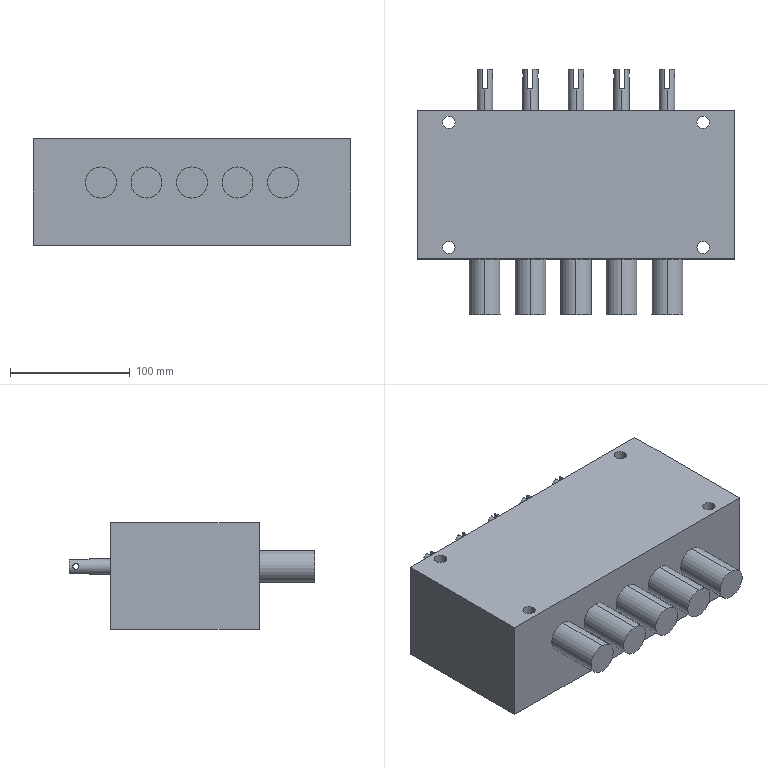Part | SolidWorks | features ICE 5, LPattern 4, Extrusion 1, RefAxis 1 | 1 solid | 84 faces | box 266 x 205.5 x 88.9 mm | volume 3043785 mm3 | cylinder 48 | plane 36 | commonest cylinder face diameters 4.88 x20 13 x10 26 x10 10.4 x8